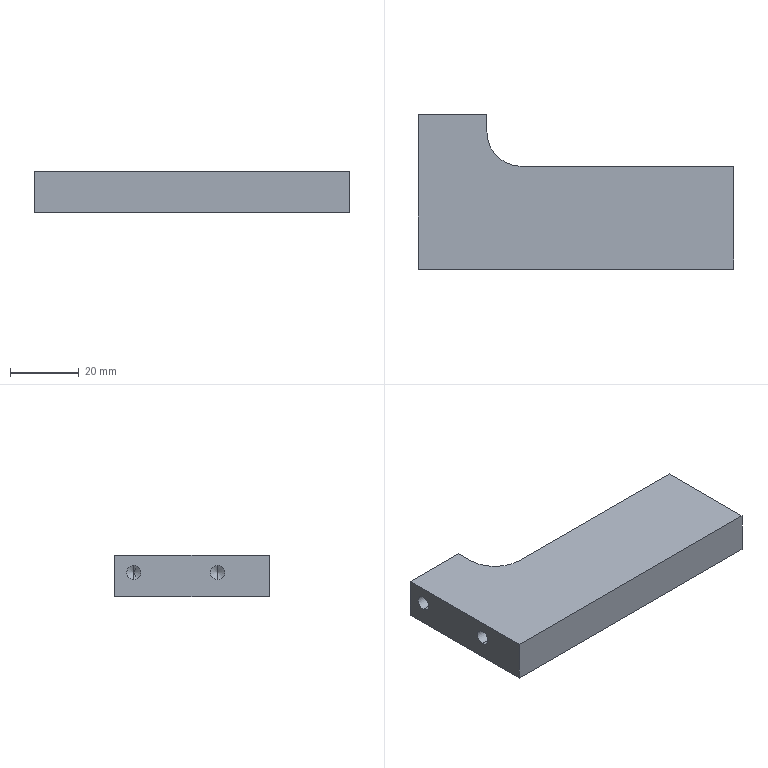Part | NX | features BREP 1 | 1 solid | 29 faces | box 92 x 45 x 12 mm | volume 35924 mm3 | cylinder 11 | cone 10 | plane 8 | commonest cylinder face diameters 4.2 x4 5 x4 3.3 x2 20 x1
STEP:
#1=CARTESIAN_POINT('',(-666.312,27.77,8.5));
#2=VERTEX_POINT('',#1);
#3=CARTESIAN_POINT('',(-666.312,27.77,3.5));
#4=VERTEX_POINT('',#3);
#5=CARTESIAN_POINT('',(-666.312,27.77,6.));
#6=DIRECTION('',(1.,0.,0.));
#7=DIRECTION('',(0.,0.,-1.));
#8=AXIS2_PLACEMENT_3D('',#5,#6,#7);
#9=CIRCLE('',#8,2.5);
#10=EDGE_CURVE('',#2,#4,#9,.T.);
#11=ORIENTED_EDGE('',*,*,#10,.F.);
#12=CARTESIAN_POINT('',(-651.312,27.77,8.5));
#13=VERTEX_POINT('',#12);
#14=CARTESIAN_POINT('',(-651.312,27.77,8.5));
#15=DIRECTION('',(1.,0.,0.));
#16=VECTOR('',#15,1000.);
#17=LINE('',#14,#16);
#18=EDGE_CURVE('',#2,#13,#17,.T.);
#19=ORIENTED_EDGE('',*,*,#18,.T.);
#20=CARTESIAN_POINT('',(-651.312,27.77,3.5));
#21=VERTEX_POINT('',#20);
#22=CARTESIAN_POINT('',(-651.312,27.77,6.));
#23=DIRECTION('',(1.,0.,0.));
#24=DIRECTION('',(0.,0.,-1.));
#25=AXIS2_PLACEMENT_3D('',#22,#23,#24);
#26=CIRCLE('',#25,2.5);
#27=EDGE_CURVE('',#13,#21,#26,.T.);
#28=ORIENTED_EDGE('',*,*,#27,.T.);
#29=CARTESIAN_POINT('',(-651.312,27.77,3.5));
#30=DIRECTION('',(1.,0.,0.));
#31=VECTOR('',#30,1000.);
#32=LINE('',#29,#31);
#33=EDGE_CURVE('',#4,#21,#32,.T.);
#34=ORIENTED_EDGE('',*,*,#33,.F.);
#35=EDGE_LOOP('',(#11,#19,#28,#34));
#36=FACE_BOUND('',#35,.T.);
#37=CARTESIAN_POINT('',(-651.312,27.77,6.));
#38=DIRECTION('',(1.,0.,0.));
#39=DIRECTION('',(0.,0.,-1.));
#40=AXIS2_PLACEMENT_3D('',#37,#38,#39);
#41=CYLINDRICAL_SURFACE('',#40,2.5);
#42=ADVANCED_FACE('',(#36),#41,.F.);
#43=CARTESIAN_POINT('',(-667.814,27.77,6.));
#44=VERTEX_POINT('',#43);
#45=CARTESIAN_POINT('',(-666.312,27.77,3.5));
#46=DIRECTION('',(0.515,0.,-0.8572));
#47=VECTOR('',#46,1000.);
#48=LINE('',#45,#47);
#49=EDGE_CURVE('',#44,#4,#48,.T.);
#50=ORIENTED_EDGE('',*,*,#49,.F.);
#51=CARTESIAN_POINT('',(-666.312,27.77,8.5));
#52=DIRECTION('',(0.515,0.,0.8572));
#53=VECTOR('',#52,1000.);
#54=LINE('',#51,#53);
#55=EDGE_CURVE('',#44,#2,#54,.T.);
#56=ORIENTED_EDGE('',*,*,#55,.T.);
#57=ORIENTED_EDGE('',*,*,#10,.T.);
#58=EDGE_LOOP('',(#50,#56,#57));
#59=FACE_BOUND('',#58,.T.);
#60=CARTESIAN_POINT('',(-666.312,27.77,6.));
#61=DIRECTION('',(1.,0.,0.));
#62=DIRECTION('',(0.,0.,-1.));
#63=AXIS2_PLACEMENT_3D('',#60,#61,#62);
#64=CONICAL_SURFACE('',#63,2.5,1.03);
#65=ADVANCED_FACE('',(#59),#64,.F.);
#66=CARTESIAN_POINT('',(-666.312,44.77,8.5));
#67=VERTEX_POINT('',#66);
#68=CARTESIAN_POINT('',(-666.312,44.77,3.5));
#69=VERTEX_POINT('',#68);
#70=CARTESIAN_POINT('',(-666.312,44.77,6.));
#71=DIRECTION('',(1.,0.,0.));
#72=DIRECTION('',(0.,0.,-1.));
#73=AXIS2_PLACEMENT_3D('',#70,#71,#72);
#74=CIRCLE('',#73,2.5);
#75=EDGE_CURVE('',#67,#69,#74,.T.);
#76=ORIENTED_EDGE('',*,*,#75,.F.);
#77=CARTESIAN_POINT('',(-651.312,44.77,8.5));
#78=VERTEX_POINT('',#77);
#79=CARTESIAN_POINT('',(-651.312,44.77,8.5));
#80=DIRECTION('',(1.,0.,0.));
#81=VECTOR('',#80,1000.);
#82=LINE('',#79,#81);
#83=EDGE_CURVE('',#67,#78,#82,.T.);
#84=ORIENTED_EDGE('',*,*,#83,.T.);
#85=CARTESIAN_POINT('',(-651.312,44.77,3.5));
#86=VERTEX_POINT('',#85);
#87=CARTESIAN_POINT('',(-651.312,44.77,6.));
#88=DIRECTION('',(1.,0.,0.));
#89=DIRECTION('',(0.,0.,-1.));
#90=AXIS2_PLACEMENT_3D('',#87,#88,#89);
#91=CIRCLE('',#90,2.5);
#92=EDGE_CURVE('',#78,#86,#91,.T.);
#93=ORIENTED_EDGE('',*,*,#92,.T.);
#94=CARTESIAN_POINT('',(-651.312,44.77,3.5));
#95=DIRECTION('',(1.,0.,0.));
#96=VECTOR('',#95,1000.);
#97=LINE('',#94,#96);
#98=EDGE_CURVE('',#69,#86,#97,.T.);
#99=ORIENTED_EDGE('',*,*,#98,.F.);
#100=EDGE_LOOP('',(#76,#84,#93,#99));
#101=FACE_BOUND('',#100,.T.);
#102=CARTESIAN_POINT('',(-651.312,44.77,6.));
#103=DIRECTION('',(1.,0.,0.));
#104=DIRECTION('',(0.,0.,-1.));
#105=AXIS2_PLACEMENT_3D('',#102,#103,#104);
#106=CYLINDRICAL_SURFACE('',#105,2.5);
#107=ADVANCED_FACE('',(#101),#106,.F.);
#108=CARTESIAN_POINT('',(-667.814,44.77,6.));
#109=VERTEX_POINT('',#108);
#110=CARTESIAN_POINT('',(-666.312,44.77,3.5));
#111=DIRECTION('',(0.515,0.,-0.8572));
#112=VECTOR('',#111,1000.);
#113=LINE('',#110,#112);
#114=EDGE_CURVE('',#109,#69,#113,.T.);
#115=ORIENTED_EDGE('',*,*,#114,.F.);
#116=CARTESIAN_POINT('',(-666.312,44.77,8.5));
#117=DIRECTION('',(0.515,0.,0.8572));
#118=VECTOR('',#117,1000.);
#119=LINE('',#116,#118);
#120=EDGE_CURVE('',#109,#67,#119,.T.);
#121=ORIENTED_EDGE('',*,*,#120,.T.);
#122=ORIENTED_EDGE('',*,*,#75,.T.);
#123=EDGE_LOOP('',(#115,#121,#122));
#124=FACE_BOUND('',#123,.T.);
#125=CARTESIAN_POINT('',(-666.312,44.77,6.));
#126=DIRECTION('',(1.,0.,0.));
#127=DIRECTION('',(0.,0.,-1.));
#128=AXIS2_PLACEMENT_3D('',#125,#126,#127);
#129=CONICAL_SURFACE('',#128,2.5,1.03);
#130=ADVANCED_FACE('',(#124),#129,.F.);
#131=CARTESIAN_POINT('',(-725.162,36.27,10.1));
#132=VERTEX_POINT('',#131);
#133=CARTESIAN_POINT('',(-728.462,36.27,10.1));
#134=VERTEX_POINT('',#133);
#135=CARTESIAN_POINT('',(-726.812,36.27,10.1));
#136=DIRECTION('',(0.,0.,-1.));
#137=DIRECTION('',(-1.,0.,0.));
#138=AXIS2_PLACEMENT_3D('',#135,#136,#137);
#139=CIRCLE('',#138,1.65);
#140=EDGE_CURVE('',#132,#134,#139,.T.);
#141=ORIENTED_EDGE('',*,*,#140,.F.);
#142=CARTESIAN_POINT('',(-725.162,36.27,0.));
#143=VERTEX_POINT('',#142);
#144=CARTESIAN_POINT('',(-725.162,36.27,0.));
#145=DIRECTION('',(0.,0.,-1.));
#146=VECTOR('',#145,1000.);
#147=LINE('',#144,#146);
#148=EDGE_CURVE('',#132,#143,#147,.T.);
#149=ORIENTED_EDGE('',*,*,#148,.T.);
#150=CARTESIAN_POINT('',(-728.462,36.27,0.));
#151=VERTEX_POINT('',#150);
#152=CARTESIAN_POINT('',(-726.812,36.27,0.));
#153=DIRECTION('',(0.,0.,-1.));
#154=DIRECTION('',(-1.,0.,0.));
#155=AXIS2_PLACEMENT_3D('',#152,#153,#154);
#156=CIRCLE('',#155,1.65);
#157=EDGE_CURVE('',#143,#151,#156,.T.);
#158=ORIENTED_EDGE('',*,*,#157,.T.);
#159=CARTESIAN_POINT('',(-728.462,36.27,0.));
#160=DIRECTION('',(0.,0.,-1.));
#161=VECTOR('',#160,1000.);
#162=LINE('',#159,#161);
#163=EDGE_CURVE('',#134,#151,#162,.T.);
#164=ORIENTED_EDGE('',*,*,#163,.F.);
#165=EDGE_LOOP('',(#141,#149,#158,#164));
#166=FACE_BOUND('',#165,.T.);
#167=CARTESIAN_POINT('',(-726.812,36.27,0.));
#168=DIRECTION('',(0.,0.,-1.));
#169=DIRECTION('',(-1.,0.,0.));
#170=AXIS2_PLACEMENT_3D('',#167,#168,#169);
#171=CYLINDRICAL_SURFACE('',#170,1.65);
#172=ADVANCED_FACE('',(#166),#171,.F.);
#173=CARTESIAN_POINT('',(-726.812,36.27,11.091));
#174=VERTEX_POINT('',#173);
#175=CARTESIAN_POINT('',(-728.462,36.27,10.1));
#176=DIRECTION('',(-0.8572,0.,-0.515));
#177=VECTOR('',#176,1000.);
#178=LINE('',#175,#177);
#179=EDGE_CURVE('',#174,#134,#178,.T.);
#180=ORIENTED_EDGE('',*,*,#179,.F.);
#181=CARTESIAN_POINT('',(-725.162,36.27,10.1));
#182=DIRECTION('',(0.8572,0.,-0.515));
#183=VECTOR('',#182,1000.);
#184=LINE('',#181,#183);
#185=EDGE_CURVE('',#174,#132,#184,.T.);
#186=ORIENTED_EDGE('',*,*,#185,.T.);
#187=ORIENTED_EDGE('',*,*,#140,.T.);
#188=EDGE_LOOP('',(#180,#186,#187));
#189=FACE_BOUND('',#188,.T.);
#190=CARTESIAN_POINT('',(-726.812,36.27,10.1));
#191=DIRECTION('',(0.,0.,-1.));
#192=DIRECTION('',(-1.,0.,0.));
#193=AXIS2_PLACEMENT_3D('',#190,#191,#192);
#194=CONICAL_SURFACE('',#193,1.65,1.03);
#195=ADVANCED_FACE('',(#189),#194,.F.);
#196=CARTESIAN_POINT('',(-730.912,36.27,4.9));
#197=VERTEX_POINT('',#196);
#198=CARTESIAN_POINT('',(-730.912,36.27,9.1));
#199=VERTEX_POINT('',#198);
#200=CARTESIAN_POINT('',(-730.912,36.27,7.));
#201=DIRECTION('',(-1.,0.,0.));
#202=DIRECTION('',(0.,0.,1.));
#203=AXIS2_PLACEMENT_3D('',#200,#201,#202);
#204=CIRCLE('',#203,2.1);
#205=EDGE_CURVE('',#197,#199,#204,.T.);
#206=ORIENTED_EDGE('',*,*,#205,.F.);
#207=CARTESIAN_POINT('',(-743.312,36.27,4.9));
#208=VERTEX_POINT('',#207);
#209=CARTESIAN_POINT('',(-743.312,36.27,4.9));
#210=DIRECTION('',(-1.,0.,0.));
#211=VECTOR('',#210,1000.);
#212=LINE('',#209,#211);
#213=EDGE_CURVE('',#208,#197,#212,.F.);
#214=ORIENTED_EDGE('',*,*,#213,.F.);
#215=CARTESIAN_POINT('',(-743.312,36.27,9.1));
#216=VERTEX_POINT('',#215);
#217=CARTESIAN_POINT('',(-743.312,36.27,7.));
#218=DIRECTION('',(-1.,0.,0.));
#219=DIRECTION('',(0.,0.,1.));
#220=AXIS2_PLACEMENT_3D('',#217,#218,#219);
#221=CIRCLE('',#220,2.1);
#222=EDGE_CURVE('',#208,#216,#221,.T.);
#223=ORIENTED_EDGE('',*,*,#222,.T.);
#224=CARTESIAN_POINT('',(-743.312,36.27,9.1));
#225=DIRECTION('',(-1.,0.,0.));
#226=VECTOR('',#225,1000.);
#227=LINE('',#224,#226);
#228=EDGE_CURVE('',#216,#199,#227,.F.);
#229=ORIENTED_EDGE('',*,*,#228,.T.);
#230=EDGE_LOOP('',(#206,#214,#223,#229));
#231=FACE_BOUND('',#230,.T.);
#232=CARTESIAN_POINT('',(-743.312,36.27,7.));
#233=DIRECTION('',(-1.,0.,0.));
#234=DIRECTION('',(0.,0.,1.));
#235=AXIS2_PLACEMENT_3D('',#232,#233,#234);
#236=CYLINDRICAL_SURFACE('',#235,2.1);
#237=ADVANCED_FACE('',(#231),#236,.F.);
#238=CARTESIAN_POINT('',(-729.65,36.27,7.));
#239=VERTEX_POINT('',#238);
#240=CARTESIAN_POINT('',(-730.912,36.27,9.1));
#241=DIRECTION('',(-0.515,0.,0.8572));
#242=VECTOR('',#241,1000.);
#243=LINE('',#240,#242);
#244=EDGE_CURVE('',#199,#239,#243,.F.);
#245=ORIENTED_EDGE('',*,*,#244,.T.);
#246=CARTESIAN_POINT('',(-730.912,36.27,4.9));
#247=DIRECTION('',(-0.515,0.,-0.8572));
#248=VECTOR('',#247,1000.);
#249=LINE('',#246,#248);
#250=EDGE_CURVE('',#197,#239,#249,.F.);
#251=ORIENTED_EDGE('',*,*,#250,.F.);
#252=ORIENTED_EDGE('',*,*,#205,.T.);
#253=EDGE_LOOP('',(#245,#251,#252));
#254=FACE_BOUND('',#253,.T.);
#255=CARTESIAN_POINT('',(-730.912,36.27,7.));
#256=DIRECTION('',(-1.,0.,0.));
#257=DIRECTION('',(0.,0.,1.));
#258=AXIS2_PLACEMENT_3D('',#255,#256,#257);
#259=CONICAL_SURFACE('',#258,2.1,1.03);
#260=ADVANCED_FACE('',(#254),#259,.F.);
#261=CARTESIAN_POINT('',(-730.912,60.77,4.9));
#262=VERTEX_POINT('',#261);
#263=CARTESIAN_POINT('',(-730.912,60.77,9.1));
#264=VERTEX_POINT('',#263);
#265=CARTESIAN_POINT('',(-730.912,60.77,7.));
#266=DIRECTION('',(-1.,0.,0.));
#267=DIRECTION('',(0.,0.,1.));
#268=AXIS2_PLACEMENT_3D('',#265,#266,#267);
#269=CIRCLE('',#268,2.1);
#270=EDGE_CURVE('',#262,#264,#269,.T.);
#271=ORIENTED_EDGE('',*,*,#270,.F.);
#272=CARTESIAN_POINT('',(-743.312,60.77,4.9));
#273=VERTEX_POINT('',#272);
#274=CARTESIAN_POINT('',(-743.312,60.77,4.9));
#275=DIRECTION('',(-1.,0.,0.));
#276=VECTOR('',#275,1000.);
#277=LINE('',#274,#276);
#278=EDGE_CURVE('',#273,#262,#277,.F.);
#279=ORIENTED_EDGE('',*,*,#278,.F.);
#280=CARTESIAN_POINT('',(-743.312,60.77,9.1));
#281=VERTEX_POINT('',#280);
#282=CARTESIAN_POINT('',(-743.312,60.77,7.));
#283=DIRECTION('',(-1.,0.,0.));
#284=DIRECTION('',(0.,0.,1.));
#285=AXIS2_PLACEMENT_3D('',#282,#283,#284);
#286=CIRCLE('',#285,2.1);
#287=EDGE_CURVE('',#273,#281,#286,.T.);
#288=ORIENTED_EDGE('',*,*,#287,.T.);
#289=CARTESIAN_POINT('',(-743.312,60.77,9.1));
#290=DIRECTION('',(-1.,0.,0.));
#291=VECTOR('',#290,1000.);
#292=LINE('',#289,#291);
#293=EDGE_CURVE('',#281,#264,#292,.F.);
#294=ORIENTED_EDGE('',*,*,#293,.T.);
#295=EDGE_LOOP('',(#271,#279,#288,#294));
#296=FACE_BOUND('',#295,.T.);
#297=CARTESIAN_POINT('',(-743.312,60.77,7.));
#298=DIRECTION('',(-1.,0.,0.));
#299=DIRECTION('',(0.,0.,1.));
#300=AXIS2_PLACEMENT_3D('',#297,#298,#299);
#301=CYLINDRICAL_SURFACE('',#300,2.1);
#302=ADVANCED_FACE('',(#296),#301,.F.);
#303=CARTESIAN_POINT('',(-729.65,60.77,7.));
#304=VERTEX_POINT('',#303);
#305=CARTESIAN_POINT('',(-730.912,60.77,9.1));
#306=DIRECTION('',(-0.515,0.,0.8572));
#307=VECTOR('',#306,1000.);
#308=LINE('',#305,#307);
#309=EDGE_CURVE('',#264,#304,#308,.F.);
#310=ORIENTED_EDGE('',*,*,#309,.T.);
#311=CARTESIAN_POINT('',(-730.912,60.77,4.9));
#312=DIRECTION('',(-0.515,0.,-0.8572));
#313=VECTOR('',#312,1000.);
#314=LINE('',#311,#313);
#315=EDGE_CURVE('',#262,#304,#314,.F.);
#316=ORIENTED_EDGE('',*,*,#315,.F.);
#317=ORIENTED_EDGE('',*,*,#270,.T.);
#318=EDGE_LOOP('',(#310,#316,#317));
#319=FACE_BOUND('',#318,.T.);
#320=CARTESIAN_POINT('',(-730.912,60.77,7.));
#321=DIRECTION('',(-1.,0.,0.));
#322=DIRECTION('',(0.,0.,1.));
#323=AXIS2_PLACEMENT_3D('',#320,#321,#322);
#324=CONICAL_SURFACE('',#323,2.1,1.03);
#325=ADVANCED_FACE('',(#319),#324,.F.);
#326=CARTESIAN_POINT('',(-651.312,51.27,0.));
#327=VERTEX_POINT('',#326);
#328=CARTESIAN_POINT('',(-713.312,51.27,0.));
#329=VERTEX_POINT('',#328);
#330=CARTESIAN_POINT('',(-743.312,51.27,0.));
#331=DIRECTION('',(-1.,0.,0.));
#332=VECTOR('',#331,1000.);
#333=LINE('',#330,#332);
#334=EDGE_CURVE('',#327,#329,#333,.T.);
#335=ORIENTED_EDGE('',*,*,#334,.T.);
#336=CARTESIAN_POINT('',(-713.312,51.27,12.));
#337=VERTEX_POINT('',#336);
#338=CARTESIAN_POINT('',(-713.312,51.27,12.));
#339=DIRECTION('',(0.,0.,1.));
#340=VECTOR('',#339,1000.);
#341=LINE('',#338,#340);
#342=EDGE_CURVE('',#329,#337,#341,.T.);
#343=ORIENTED_EDGE('',*,*,#342,.T.);
#344=CARTESIAN_POINT('',(-651.312,51.27,12.));
#345=VERTEX_POINT('',#344);
#346=CARTESIAN_POINT('',(-743.312,51.27,12.));
#347=DIRECTION('',(-1.,0.,0.));
#348=VECTOR('',#347,1000.);
#349=LINE('',#346,#348);
#350=EDGE_CURVE('',#345,#337,#349,.T.);
#351=ORIENTED_EDGE('',*,*,#350,.F.);
#352=CARTESIAN_POINT('',(-651.312,51.27,12.));
#353=DIRECTION('',(0.,0.,-1.));
#354=VECTOR('',#353,1000.);
#355=LINE('',#352,#354);
#356=EDGE_CURVE('',#345,#327,#355,.T.);
#357=ORIENTED_EDGE('',*,*,#356,.T.);
#358=EDGE_LOOP('',(#335,#343,#351,#357));
#359=FACE_BOUND('',#358,.T.);
#360=CARTESIAN_POINT('',(-743.312,51.27,12.));
#361=DIRECTION('',(0.,-1.,0.));
#362=DIRECTION('',(0.,0.,-1.));
#363=AXIS2_PLACEMENT_3D('',#360,#361,#362);
#364=PLANE('',#363);
#365=ADVANCED_FACE('',(#359),#364,.F.);
#366=CARTESIAN_POINT('',(-743.312,66.27,0.));
#367=VERTEX_POINT('',#366);
#368=CARTESIAN_POINT('',(-743.312,21.27,0.));
#369=VERTEX_POINT('',#368);
#370=CARTESIAN_POINT('',(-743.312,21.27,0.));
#371=DIRECTION('',(0.,-1.,0.));
#372=VECTOR('',#371,1000.);
#373=LINE('',#370,#372);
#374=EDGE_CURVE('',#367,#369,#373,.T.);
#375=ORIENTED_EDGE('',*,*,#374,.T.);
#376=CARTESIAN_POINT('',(-743.312,21.27,12.));
#377=VERTEX_POINT('',#376);
#378=CARTESIAN_POINT('',(-743.312,21.27,12.));
#379=DIRECTION('',(0.,0.,-1.));
#380=VECTOR('',#379,1000.);
#381=LINE('',#378,#380);
#382=EDGE_CURVE('',#377,#369,#381,.T.);
#383=ORIENTED_EDGE('',*,*,#382,.F.);
#384=CARTESIAN_POINT('',(-743.312,66.27,12.));
#385=VERTEX_POINT('',#384);
#386=CARTESIAN_POINT('',(-743.312,21.27,12.));
#387=DIRECTION('',(0.,-1.,0.));
#388=VECTOR('',#387,1000.);
#389=LINE('',#386,#388);
#390=EDGE_CURVE('',#385,#377,#389,.T.);
#391=ORIENTED_EDGE('',*,*,#390,.F.);
#392=CARTESIAN_POINT('',(-743.312,66.27,12.));
#393=DIRECTION('',(0.,0.,1.));
#394=VECTOR('',#393,1000.);
#395=LINE('',#392,#394);
#396=EDGE_CURVE('',#367,#385,#395,.T.);
#397=ORIENTED_EDGE('',*,*,#396,.F.);
#398=EDGE_LOOP('',(#375,#383,#391,#397));
#399=FACE_BOUND('',#398,.T.);
#400=CARTESIAN_POINT('',(-743.312,36.27,7.));
#401=DIRECTION('',(-1.,0.,0.));
#402=DIRECTION('',(0.,0.,1.));
#403=AXIS2_PLACEMENT_3D('',#400,#401,#402);
#404=CIRCLE('',#403,2.1);
#405=EDGE_CURVE('',#216,#208,#404,.T.);
#406=ORIENTED_EDGE('',*,*,#405,.F.);
#407=ORIENTED_EDGE('',*,*,#222,.F.);
#408=EDGE_LOOP('',(#406,#407));
#409=FACE_BOUND('',#408,.T.);
#410=CARTESIAN_POINT('',(-743.312,60.77,7.));
#411=DIRECTION('',(-1.,0.,0.));
#412=DIRECTION('',(0.,0.,1.));
#413=AXIS2_PLACEMENT_3D('',#410,#411,#412);
#414=CIRCLE('',#413,2.1);
#415=EDGE_CURVE('',#281,#273,#414,.T.);
#416=ORIENTED_EDGE('',*,*,#415,.F.);
#417=ORIENTED_EDGE('',*,*,#287,.F.);
#418=EDGE_LOOP('',(#416,#417));
#419=FACE_BOUND('',#418,.T.);
#420=CARTESIAN_POINT('',(-743.312,21.27,12.));
#421=DIRECTION('',(1.,0.,0.));
#422=DIRECTION('',(0.,1.,0.));
#423=AXIS2_PLACEMENT_3D('',#420,#421,#422);
#424=PLANE('',#423);
#425=ADVANCED_FACE('',(#399,#409,#419),#424,.F.);
#426=CARTESIAN_POINT('',(-651.312,21.27,0.));
#427=VERTEX_POINT('',#426);
#428=CARTESIAN_POINT('',(-743.312,21.27,0.));
#429=DIRECTION('',(1.,0.,0.));
#430=VECTOR('',#429,1000.);
#431=LINE('',#428,#430);
#432=EDGE_CURVE('',#369,#427,#431,.T.);
#433=ORIENTED_EDGE('',*,*,#432,.T.);
#434=CARTESIAN_POINT('',(-651.312,21.27,12.));
#435=VERTEX_POINT('',#434);
#436=CARTESIAN_POINT('',(-651.312,21.27,12.));
#437=DIRECTION('',(0.,0.,-1.));
#438=VECTOR('',#437,1000.);
#439=LINE('',#436,#438);
#440=EDGE_CURVE('',#435,#427,#439,.T.);
#441=ORIENTED_EDGE('',*,*,#440,.F.);
#442=CARTESIAN_POINT('',(-743.312,21.27,12.));
#443=DIRECTION('',(1.,0.,0.));
#444=VECTOR('',#443,1000.);
#445=LINE('',#442,#444);
#446=EDGE_CURVE('',#377,#435,#445,.T.);
#447=ORIENTED_EDGE('',*,*,#446,.F.);
#448=ORIENTED_EDGE('',*,*,#382,.T.);
#449=EDGE_LOOP('',(#433,#441,#447,#448));
#450=FACE_BOUND('',#449,.T.);
#451=CARTESIAN_POINT('',(-743.312,21.27,12.));
#452=DIRECTION('',(0.,1.,0.));
#453=DIRECTION('',(1.,0.,0.));
#454=AXIS2_PLACEMENT_3D('',#451,#452,#453);
#455=PLANE('',#454);
#456=ADVANCED_FACE('',(#450),#455,.F.);
#457=CARTESIAN_POINT('',(-651.312,21.27,0.));
#458=DIRECTION('',(0.,1.,0.));
#459=VECTOR('',#458,1000.);
#460=LINE('',#457,#459);
#461=EDGE_CURVE('',#427,#327,#460,.T.);
#462=ORIENTED_EDGE('',*,*,#461,.T.);
#463=ORIENTED_EDGE('',*,*,#356,.F.);
#464=CARTESIAN_POINT('',(-651.312,21.27,12.));
#465=DIRECTION('',(0.,1.,0.));
#466=VECTOR('',#465,1000.);
#467=LINE('',#464,#466);
#468=EDGE_CURVE('',#435,#345,#467,.T.);
#469=ORIENTED_EDGE('',*,*,#468,.F.);
#470=ORIENTED_EDGE('',*,*,#440,.T.);
#471=EDGE_LOOP('',(#462,#463,#469,#470));
#472=FACE_BOUND('',#471,.T.);
#473=CARTESIAN_POINT('',(-651.312,27.77,6.));
#474=DIRECTION('',(1.,0.,0.));
#475=DIRECTION('',(0.,0.,-1.));
#476=AXIS2_PLACEMENT_3D('',#473,#474,#475);
#477=CIRCLE('',#476,2.5);
#478=EDGE_CURVE('',#21,#13,#477,.T.);
#479=ORIENTED_EDGE('',*,*,#478,.F.);
#480=ORIENTED_EDGE('',*,*,#27,.F.);
#481=EDGE_LOOP('',(#479,#480));
#482=FACE_BOUND('',#481,.T.);
#483=CARTESIAN_POINT('',(-651.312,44.77,6.));
#484=DIRECTION('',(1.,0.,0.));
#485=DIRECTION('',(0.,0.,-1.));
#486=AXIS2_PLACEMENT_3D('',#483,#484,#485);
#487=CIRCLE('',#486,2.5);
#488=EDGE_CURVE('',#86,#78,#487,.T.);
#489=ORIENTED_EDGE('',*,*,#488,.F.);
#490=ORIENTED_EDGE('',*,*,#92,.F.);
#491=EDGE_LOOP('',(#489,#490));
#492=FACE_BOUND('',#491,.T.);
#493=CARTESIAN_POINT('',(-651.312,21.27,12.));
#494=DIRECTION('',(-1.,0.,0.));
#495=DIRECTION('',(0.,0.,1.));
#496=AXIS2_PLACEMENT_3D('',#493,#494,#495);
#497=PLANE('',#496);
#498=ADVANCED_FACE('',(#472,#482,#492),#497,.F.);
#499=ORIENTED_EDGE('',*,*,#390,.T.);
#500=ORIENTED_EDGE('',*,*,#446,.T.);
#501=ORIENTED_EDGE('',*,*,#468,.T.);
#502=ORIENTED_EDGE('',*,*,#350,.T.);
#503=CARTESIAN_POINT('',(-723.312,61.27,12.));
#504=VERTEX_POINT('',#503);
#505=CARTESIAN_POINT('',(-713.312,61.27,12.));
#506=DIRECTION('',(0.,0.,-1.));
#507=DIRECTION('',(-1.,0.,0.));
#508=AXIS2_PLACEMENT_3D('',#505,#506,#507);
#509=CIRCLE('',#508,10.);
#510=EDGE_CURVE('',#337,#504,#509,.T.);
#511=ORIENTED_EDGE('',*,*,#510,.T.);
#512=CARTESIAN_POINT('',(-723.312,66.27,12.));
#513=VERTEX_POINT('',#512);
#514=CARTESIAN_POINT('',(-723.312,66.27,12.));
#515=DIRECTION('',(0.,-1.,0.));
#516=VECTOR('',#515,1000.);
#517=LINE('',#514,#516);
#518=EDGE_CURVE('',#513,#504,#517,.T.);
#519=ORIENTED_EDGE('',*,*,#518,.F.);
#520=CARTESIAN_POINT('',(-743.312,66.27,12.));
#521=DIRECTION('',(1.,0.,0.));
#522=VECTOR('',#521,1000.);
#523=LINE('',#520,#522);
#524=EDGE_CURVE('',#385,#513,#523,.T.);
#525=ORIENTED_EDGE('',*,*,#524,.F.);
#526=EDGE_LOOP('',(#499,#500,#501,#502,#511,#519,#525));
#527=FACE_BOUND('',#526,.T.);
#528=CARTESIAN_POINT('',(-743.312,51.27,12.));
#529=DIRECTION('',(0.,0.,-1.));
#530=DIRECTION('',(0.,-1.,0.));
#531=AXIS2_PLACEMENT_3D('',#528,#529,#530);
#532=PLANE('',#531);
#533=ADVANCED_FACE('',(#527),#532,.F.);
#534=ORIENTED_EDGE('',*,*,#374,.F.);
#535=CARTESIAN_POINT('',(-723.312,66.27,0.));
#536=VERTEX_POINT('',#535);
#537=CARTESIAN_POINT('',(-743.312,66.27,0.));
#538=DIRECTION('',(-1.,0.,0.));
#539=VECTOR('',#538,1000.);
#540=LINE('',#537,#539);
#541=EDGE_CURVE('',#536,#367,#540,.T.);
#542=ORIENTED_EDGE('',*,*,#541,.F.);
#543=CARTESIAN_POINT('',(-723.312,61.27,0.));
#544=VERTEX_POINT('',#543);
#545=CARTESIAN_POINT('',(-723.312,66.27,0.));
#546=DIRECTION('',(0.,-1.,0.));
#547=VECTOR('',#546,1000.);
#548=LINE('',#545,#547);
#549=EDGE_CURVE('',#536,#544,#548,.T.);
#550=ORIENTED_EDGE('',*,*,#549,.T.);
#551=CARTESIAN_POINT('',(-713.312,61.27,0.));
#552=DIRECTION('',(0.,0.,1.));
#553=DIRECTION('',(-1.,0.,0.));
#554=AXIS2_PLACEMENT_3D('',#551,#552,#553);
#555=CIRCLE('',#554,10.);
#556=EDGE_CURVE('',#544,#329,#555,.T.);
#557=ORIENTED_EDGE('',*,*,#556,.T.);
#558=ORIENTED_EDGE('',*,*,#334,.F.);
#559=ORIENTED_EDGE('',*,*,#461,.F.);
#560=ORIENTED_EDGE('',*,*,#432,.F.);
#561=EDGE_LOOP('',(#534,#542,#550,#557,#558,#559,#560));
#562=FACE_BOUND('',#561,.T.);
#563=CARTESIAN_POINT('',(-726.812,36.27,0.));
#564=DIRECTION('',(0.,0.,-1.));
#565=DIRECTION('',(-1.,0.,0.));
#566=AXIS2_PLACEMENT_3D('',#563,#564,#565);
#567=CIRCLE('',#566,1.65);
#568=EDGE_CURVE('',#151,#143,#567,.T.);
#569=ORIENTED_EDGE('',*,*,#568,.F.);
#570=ORIENTED_EDGE('',*,*,#157,.F.);
#571=EDGE_LOOP('',(#569,#570));
#572=FACE_BOUND('',#571,.T.);
#573=CARTESIAN_POINT('',(-743.312,51.27,0.));
#574=DIRECTION('',(0.,0.,-1.));
#575=DIRECTION('',(0.,-1.,0.));
#576=AXIS2_PLACEMENT_3D('',#573,#574,#575);
#577=PLANE('',#576);
#578=ADVANCED_FACE('',(#562,#572),#577,.T.);
#579=ORIENTED_EDGE('',*,*,#518,.T.);
#580=CARTESIAN_POINT('',(-723.312,61.27,0.));
#581=DIRECTION('',(0.,0.,-1.));
#582=VECTOR('',#581,1000.);
#583=LINE('',#580,#582);
#584=EDGE_CURVE('',#504,#544,#583,.T.);
#585=ORIENTED_EDGE('',*,*,#584,.T.);
#586=ORIENTED_EDGE('',*,*,#549,.F.);
#587=CARTESIAN_POINT('',(-723.312,66.27,12.));
#588=DIRECTION('',(0.,0.,-1.));
#589=VECTOR('',#588,1000.);
#590=LINE('',#587,#589);
#591=EDGE_CURVE('',#513,#536,#590,.T.);
#592=ORIENTED_EDGE('',*,*,#591,.F.);
#593=EDGE_LOOP('',(#579,#585,#586,#592));
#594=FACE_BOUND('',#593,.T.);
#595=CARTESIAN_POINT('',(-723.312,66.27,12.));
#596=DIRECTION('',(-1.,0.,0.));
#597=DIRECTION('',(0.,0.,1.));
#598=AXIS2_PLACEMENT_3D('',#595,#596,#597);
#599=PLANE('',#598);
#600=ADVANCED_FACE('',(#594),#599,.F.);
#601=ORIENTED_EDGE('',*,*,#396,.T.);
#602=ORIENTED_EDGE('',*,*,#524,.T.);
#603=ORIENTED_EDGE('',*,*,#591,.T.);
#604=ORIENTED_EDGE('',*,*,#541,.T.);
#605=EDGE_LOOP('',(#601,#602,#603,#604));
#606=FACE_BOUND('',#605,.T.);
#607=CARTESIAN_POINT('',(-743.312,66.27,0.));
#608=DIRECTION('',(0.,-1.,0.));
#609=DIRECTION('',(0.,0.,-1.));
#610=AXIS2_PLACEMENT_3D('',#607,#608,#609);
#611=PLANE('',#610);
#612=ADVANCED_FACE('',(#606),#611,.F.);
#613=ORIENTED_EDGE('',*,*,#510,.F.);
#614=ORIENTED_EDGE('',*,*,#342,.F.);
#615=ORIENTED_EDGE('',*,*,#556,.F.);
#616=ORIENTED_EDGE('',*,*,#584,.F.);
#617=EDGE_LOOP('',(#613,#614,#615,#616));
#618=FACE_BOUND('',#617,.T.);
#619=CARTESIAN_POINT('',(-713.312,61.27,12.));
#620=DIRECTION('',(0.,0.,1.));
#621=DIRECTION('',(1.,0.,0.));
#622=AXIS2_PLACEMENT_3D('',#619,#620,#621);
#623=CYLINDRICAL_SURFACE('',#622,10.);
#624=ADVANCED_FACE('',(#618),#623,.F.);
#625=ORIENTED_EDGE('',*,*,#315,.T.);
#626=ORIENTED_EDGE('',*,*,#309,.F.);
#627=CARTESIAN_POINT('',(-730.912,60.77,7.));
#628=DIRECTION('',(-1.,0.,0.));
#629=DIRECTION('',(0.,0.,1.));
#630=AXIS2_PLACEMENT_3D('',#627,#628,#629);
#631=CIRCLE('',#630,2.1);
#632=EDGE_CURVE('',#264,#262,#631,.T.);
#633=ORIENTED_EDGE('',*,*,#632,.T.);
#634=EDGE_LOOP('',(#625,#626,#633));
#635=FACE_BOUND('',#634,.T.);
#636=CARTESIAN_POINT('',(-730.912,60.77,7.));
#637=DIRECTION('',(-1.,0.,0.));
#638=DIRECTION('',(0.,0.,1.));
#639=AXIS2_PLACEMENT_3D('',#636,#637,#638);
#640=CONICAL_SURFACE('',#639,2.1,1.03);
#641=ADVANCED_FACE('',(#635),#640,.F.);
#642=ORIENTED_EDGE('',*,*,#278,.T.);
#643=ORIENTED_EDGE('',*,*,#632,.F.);
#644=ORIENTED_EDGE('',*,*,#293,.F.);
#645=ORIENTED_EDGE('',*,*,#415,.T.);
#646=EDGE_LOOP('',(#642,#643,#644,#645));
#647=FACE_BOUND('',#646,.T.);
#648=CARTESIAN_POINT('',(-743.312,60.77,7.));
#649=DIRECTION('',(-1.,0.,0.));
#650=DIRECTION('',(0.,0.,1.));
#651=AXIS2_PLACEMENT_3D('',#648,#649,#650);
#652=CYLINDRICAL_SURFACE('',#651,2.1);
#653=ADVANCED_FACE('',(#647),#652,.F.);
#654=ORIENTED_EDGE('',*,*,#250,.T.);
#655=ORIENTED_EDGE('',*,*,#244,.F.);
#656=CARTESIAN_POINT('',(-730.912,36.27,7.));
#657=DIRECTION('',(-1.,0.,0.));
#658=DIRECTION('',(0.,0.,1.));
#659=AXIS2_PLACEMENT_3D('',#656,#657,#658);
#660=CIRCLE('',#659,2.1);
#661=EDGE_CURVE('',#199,#197,#660,.T.);
#662=ORIENTED_EDGE('',*,*,#661,.T.);
#663=EDGE_LOOP('',(#654,#655,#662));
#664=FACE_BOUND('',#663,.T.);
#665=CARTESIAN_POINT('',(-730.912,36.27,7.));
#666=DIRECTION('',(-1.,0.,0.));
#667=DIRECTION('',(0.,0.,1.));
#668=AXIS2_PLACEMENT_3D('',#665,#666,#667);
#669=CONICAL_SURFACE('',#668,2.1,1.03);
#670=ADVANCED_FACE('',(#664),#669,.F.);
#671=ORIENTED_EDGE('',*,*,#213,.T.);
#672=ORIENTED_EDGE('',*,*,#661,.F.);
#673=ORIENTED_EDGE('',*,*,#228,.F.);
#674=ORIENTED_EDGE('',*,*,#405,.T.);
#675=EDGE_LOOP('',(#671,#672,#673,#674));
#676=FACE_BOUND('',#675,.T.);
#677=CARTESIAN_POINT('',(-743.312,36.27,7.));
#678=DIRECTION('',(-1.,0.,0.));
#679=DIRECTION('',(0.,0.,1.));
#680=AXIS2_PLACEMENT_3D('',#677,#678,#679);
#681=CYLINDRICAL_SURFACE('',#680,2.1);
#682=ADVANCED_FACE('',(#676),#681,.F.);
#683=ORIENTED_EDGE('',*,*,#185,.F.);
#684=ORIENTED_EDGE('',*,*,#179,.T.);
#685=CARTESIAN_POINT('',(-726.812,36.27,10.1));
#686=DIRECTION('',(0.,0.,-1.));
#687=DIRECTION('',(-1.,0.,0.));
#688=AXIS2_PLACEMENT_3D('',#685,#686,#687);
#689=CIRCLE('',#688,1.65);
#690=EDGE_CURVE('',#134,#132,#689,.T.);
#691=ORIENTED_EDGE('',*,*,#690,.T.);
#692=EDGE_LOOP('',(#683,#684,#691));
#693=FACE_BOUND('',#692,.T.);
#694=CARTESIAN_POINT('',(-726.812,36.27,10.1));
#695=DIRECTION('',(0.,0.,-1.));
#696=DIRECTION('',(-1.,0.,0.));
#697=AXIS2_PLACEMENT_3D('',#694,#695,#696);
#698=CONICAL_SURFACE('',#697,1.65,1.03);
#699=ADVANCED_FACE('',(#693),#698,.F.);
#700=ORIENTED_EDGE('',*,*,#148,.F.);
#701=ORIENTED_EDGE('',*,*,#690,.F.);
#702=ORIENTED_EDGE('',*,*,#163,.T.);
#703=ORIENTED_EDGE('',*,*,#568,.T.);
#704=EDGE_LOOP('',(#700,#701,#702,#703));
#705=FACE_BOUND('',#704,.T.);
#706=CARTESIAN_POINT('',(-726.812,36.27,0.));
#707=DIRECTION('',(0.,0.,-1.));
#708=DIRECTION('',(-1.,0.,0.));
#709=AXIS2_PLACEMENT_3D('',#706,#707,#708);
#710=CYLINDRICAL_SURFACE('',#709,1.65);
#711=ADVANCED_FACE('',(#705),#710,.F.);
#712=ORIENTED_EDGE('',*,*,#120,.F.);
#713=ORIENTED_EDGE('',*,*,#114,.T.);
#714=CARTESIAN_POINT('',(-666.312,44.77,6.));
#715=DIRECTION('',(1.,0.,0.));
#716=DIRECTION('',(0.,0.,-1.));
#717=AXIS2_PLACEMENT_3D('',#714,#715,#716);
#718=CIRCLE('',#717,2.5);
#719=EDGE_CURVE('',#69,#67,#718,.T.);
#720=ORIENTED_EDGE('',*,*,#719,.T.);
#721=EDGE_LOOP('',(#712,#713,#720));
#722=FACE_BOUND('',#721,.T.);
#723=CARTESIAN_POINT('',(-666.312,44.77,6.));
#724=DIRECTION('',(1.,0.,0.));
#725=DIRECTION('',(0.,0.,-1.));
#726=AXIS2_PLACEMENT_3D('',#723,#724,#725);
#727=CONICAL_SURFACE('',#726,2.5,1.03);
#728=ADVANCED_FACE('',(#722),#727,.F.);
#729=ORIENTED_EDGE('',*,*,#83,.F.);
#730=ORIENTED_EDGE('',*,*,#719,.F.);
#731=ORIENTED_EDGE('',*,*,#98,.T.);
#732=ORIENTED_EDGE('',*,*,#488,.T.);
#733=EDGE_LOOP('',(#729,#730,#731,#732));
#734=FACE_BOUND('',#733,.T.);
#735=CARTESIAN_POINT('',(-651.312,44.77,6.));
#736=DIRECTION('',(1.,0.,0.));
#737=DIRECTION('',(0.,0.,-1.));
#738=AXIS2_PLACEMENT_3D('',#735,#736,#737);
#739=CYLINDRICAL_SURFACE('',#738,2.5);
#740=ADVANCED_FACE('',(#734),#739,.F.);
#741=ORIENTED_EDGE('',*,*,#55,.F.);
#742=ORIENTED_EDGE('',*,*,#49,.T.);
#743=CARTESIAN_POINT('',(-666.312,27.77,6.));
#744=DIRECTION('',(1.,0.,0.));
#745=DIRECTION('',(0.,0.,-1.));
#746=AXIS2_PLACEMENT_3D('',#743,#744,#745);
#747=CIRCLE('',#746,2.5);
#748=EDGE_CURVE('',#4,#2,#747,.T.);
#749=ORIENTED_EDGE('',*,*,#748,.T.);
#750=EDGE_LOOP('',(#741,#742,#749));
#751=FACE_BOUND('',#750,.T.);
#752=CARTESIAN_POINT('',(-666.312,27.77,6.));
#753=DIRECTION('',(1.,0.,0.));
#754=DIRECTION('',(0.,0.,-1.));
#755=AXIS2_PLACEMENT_3D('',#752,#753,#754);
#756=CONICAL_SURFACE('',#755,2.5,1.03);
#757=ADVANCED_FACE('',(#751),#756,.F.);
#758=ORIENTED_EDGE('',*,*,#18,.F.);
#759=ORIENTED_EDGE('',*,*,#748,.F.);
#760=ORIENTED_EDGE('',*,*,#33,.T.);
#761=ORIENTED_EDGE('',*,*,#478,.T.);
#762=EDGE_LOOP('',(#758,#759,#760,#761));
#763=FACE_BOUND('',#762,.T.);
#764=CARTESIAN_POINT('',(-651.312,27.77,6.));
#765=DIRECTION('',(1.,0.,0.));
#766=DIRECTION('',(0.,0.,-1.));
#767=AXIS2_PLACEMENT_3D('',#764,#765,#766);
#768=CYLINDRICAL_SURFACE('',#767,2.5);
#769=ADVANCED_FACE('',(#763),#768,.F.);
#770=CLOSED_SHELL('',(#42,#65,#107,#130,#172,#195,#237,#260,#302,#325,#365,#425,#456,#498,#533,#578,#600,#612,#624,#641,#653,#670,#682,#699,#711,#728,#740,#757,#769));
#771=MANIFOLD_SOLID_BREP('',#770);
#772=(LENGTH_UNIT()NAMED_UNIT(*)SI_UNIT(.MILLI.,.METRE.));
#773=UNCERTAINTY_MEASURE_WITH_UNIT(LENGTH_MEASURE(0.00001),#772,'','');
#774=(NAMED_UNIT(*)PLANE_ANGLE_UNIT()SI_UNIT($,.RADIAN.));
#775=(NAMED_UNIT(*)SI_UNIT($,.STERADIAN.)SOLID_ANGLE_UNIT());
#776=(GEOMETRIC_REPRESENTATION_CONTEXT(3)GLOBAL_UNCERTAINTY_ASSIGNED_CONTEXT((#773))GLOBAL_UNIT_ASSIGNED_CONTEXT((#772,#774,#775))REPRESENTATION_CONTEXT('',''));
#777=ADVANCED_BREP_SHAPE_REPRESENTATION('',(#771),#776);